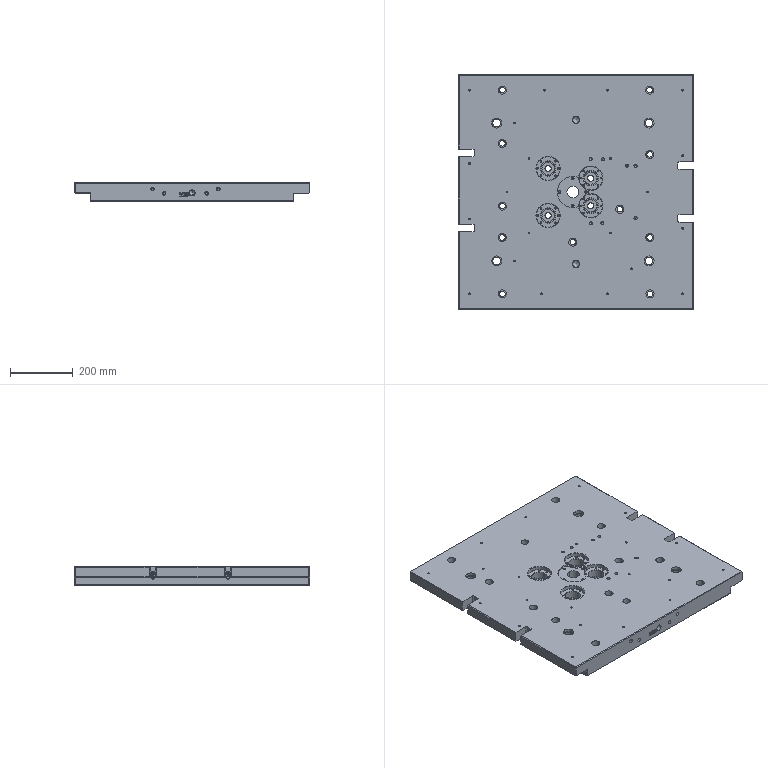Part | Creo | 1 solid | 1098 faces | box 750 x 750 x 60 mm | volume 30183757 mm3 | cylinder 472 | cone 276 | plane 207 | other 119 | torus 24 | commonest cylinder face diameters 8 x174 4.97 x42 6 x42 5.1 x32 17.5 x26 26 x22